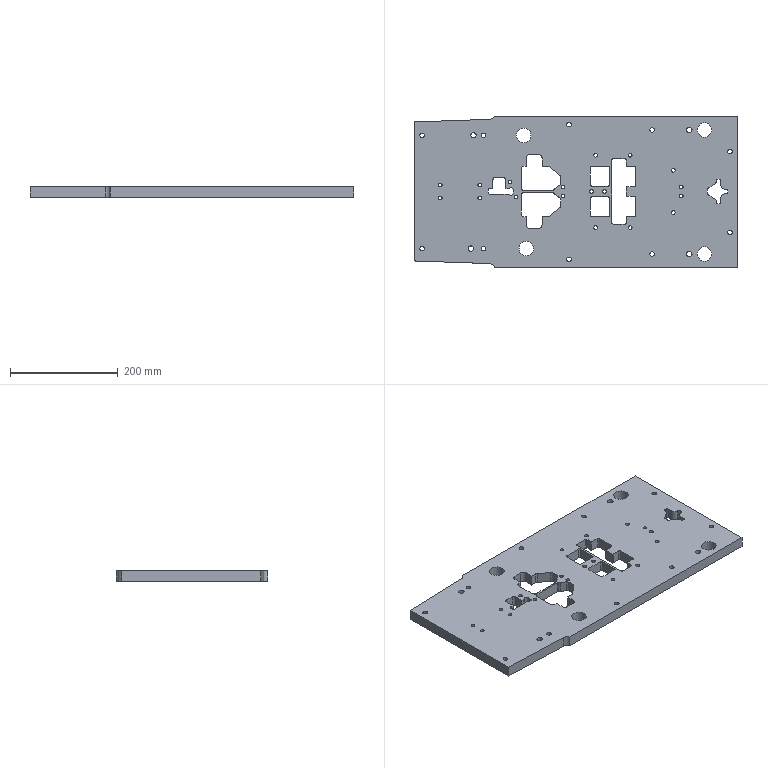Part | NX | features PPS-4 2 | 1 solid | 220 faces | box 600 x 280 x 20 mm | volume 2875043 mm3 | cylinder 117 | plane 80 | cone 17 | spline 6 | commonest cylinder face diameters 10 x26 6 x22 6.805 x11 8.5 x10 4 x8 5 x8